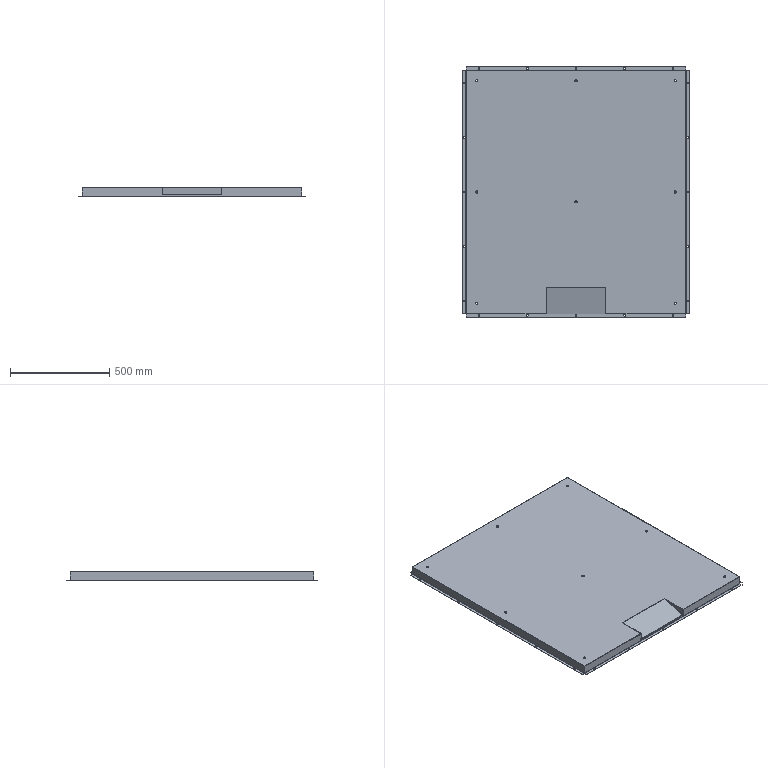Part | SolidWorks | 2 solids | 206 faces | box 1140 x 1260 x 44 mm | volume 1625232 mm3 | plane 106 | cylinder 88 | spline 12 | commonest cylinder face diameters 7 x50 11 x16 1 x9 3 x9 0.4 x2 2.4 x2